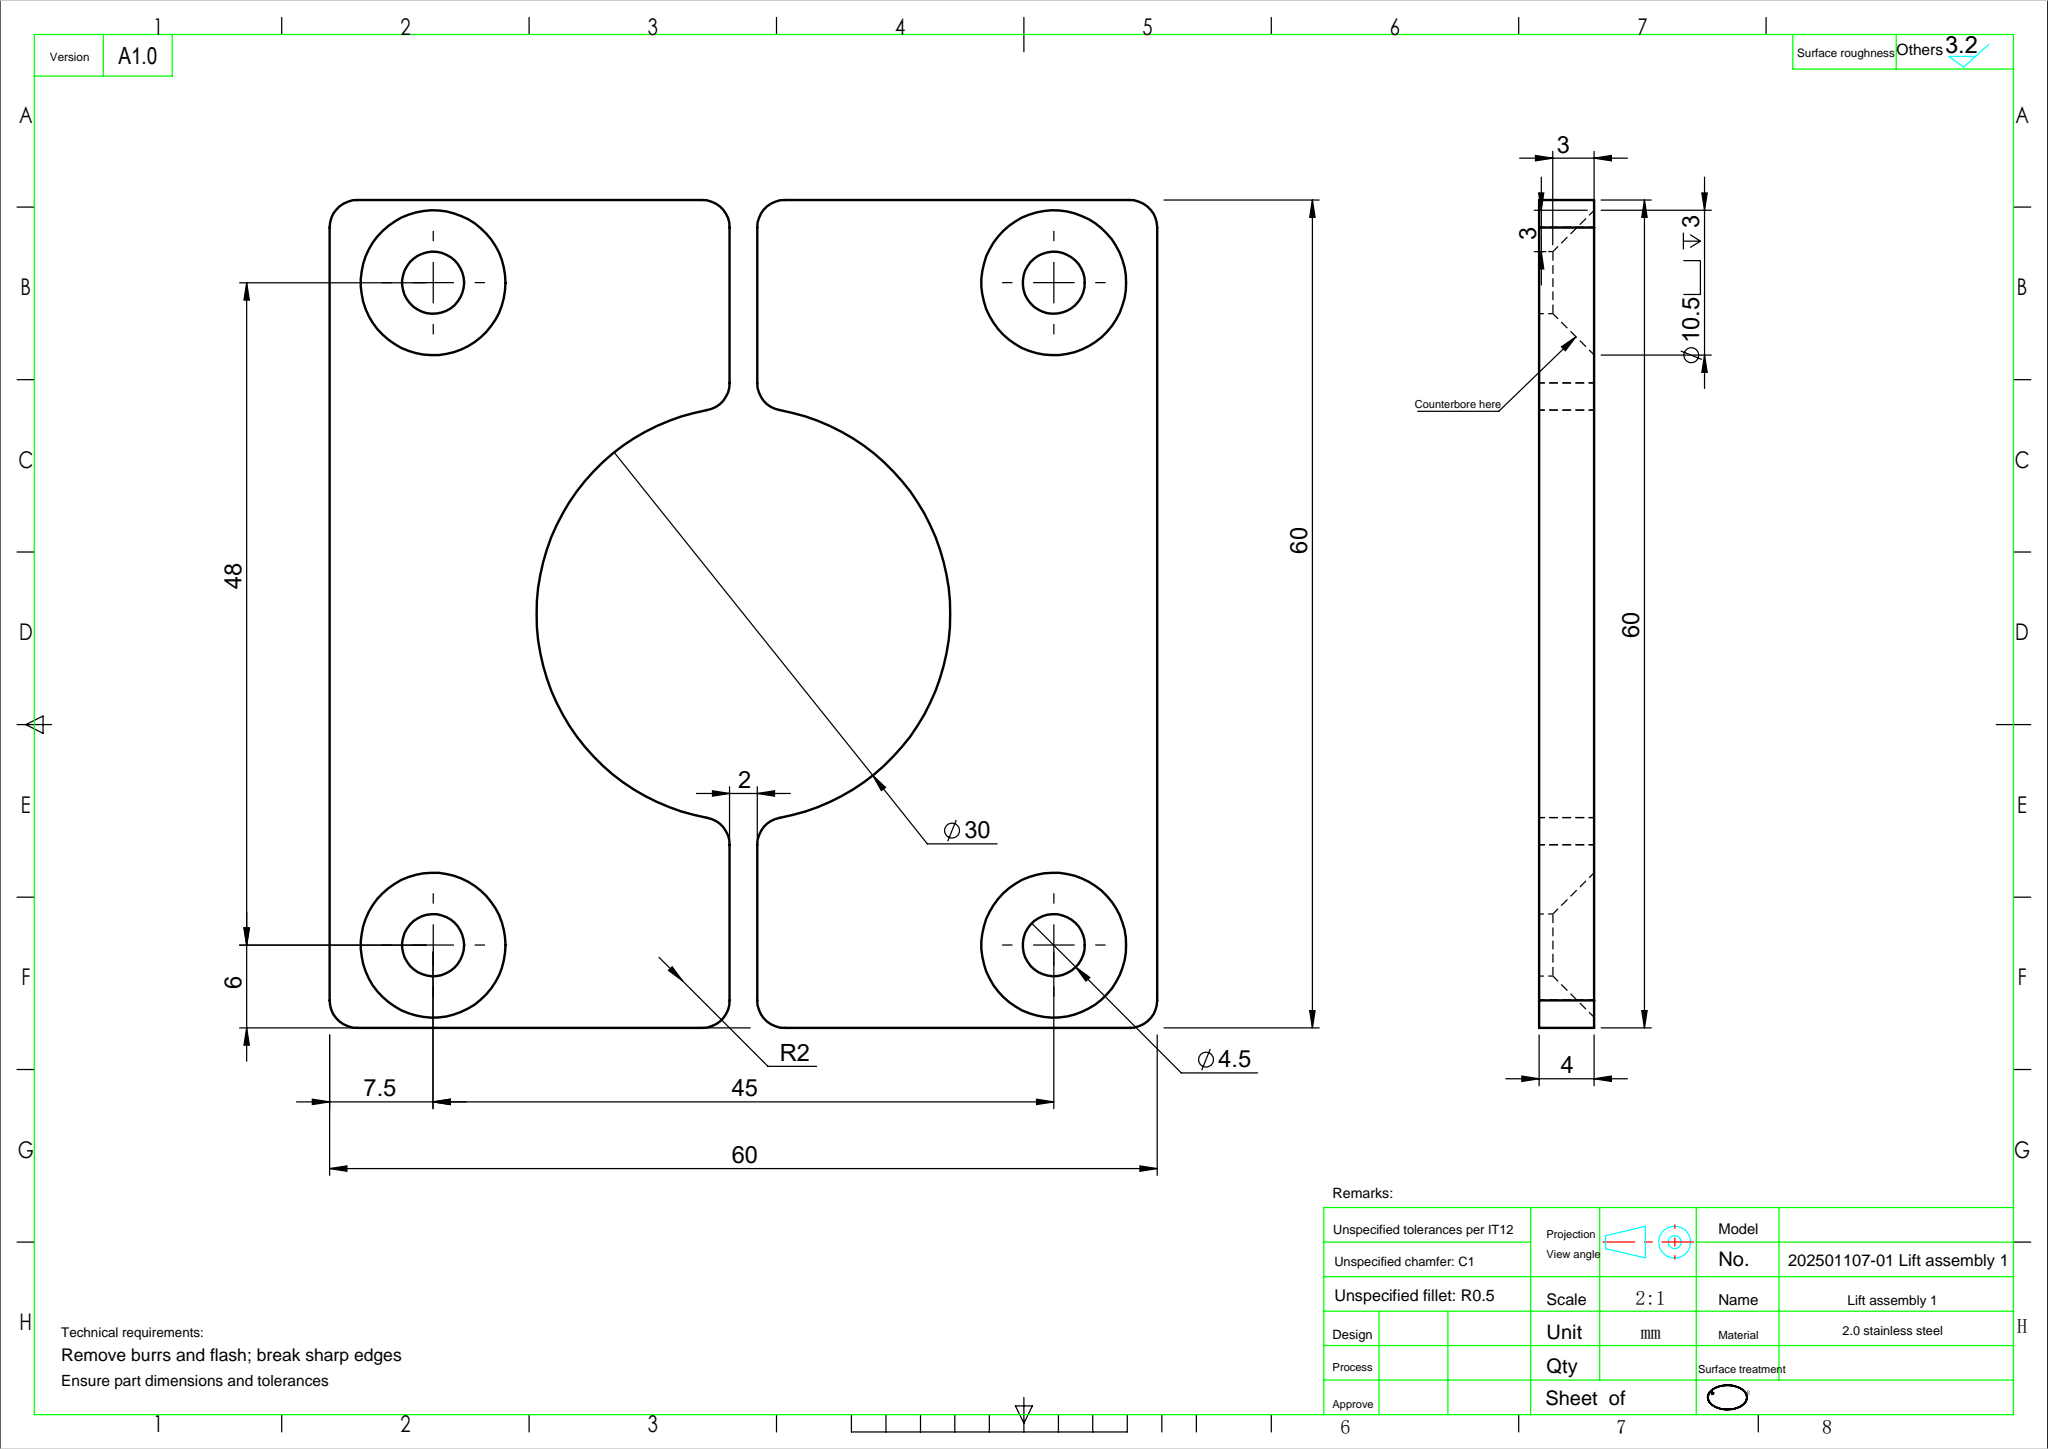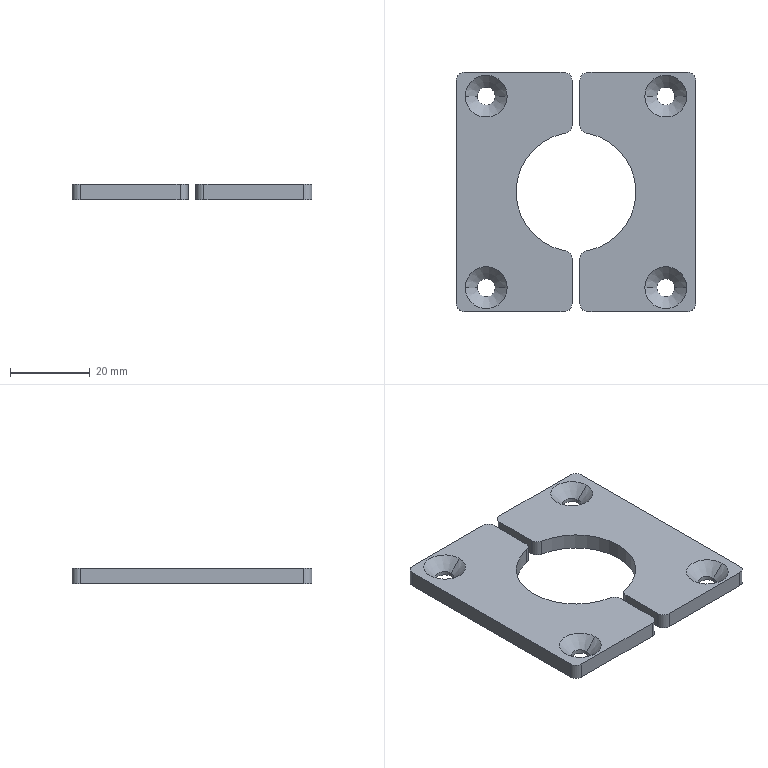Part | SolidWorks | features Chamfer 2, Fillet 2, ICE 2, Extrusion 1 | 2 solids | 45 faces | box 60 x 60 x 4 mm | volume 10673 mm3 | cylinder 23 | plane 14 | cone 8 | commonest cylinder face diameters 4 x12 4.5 x8 30 x3